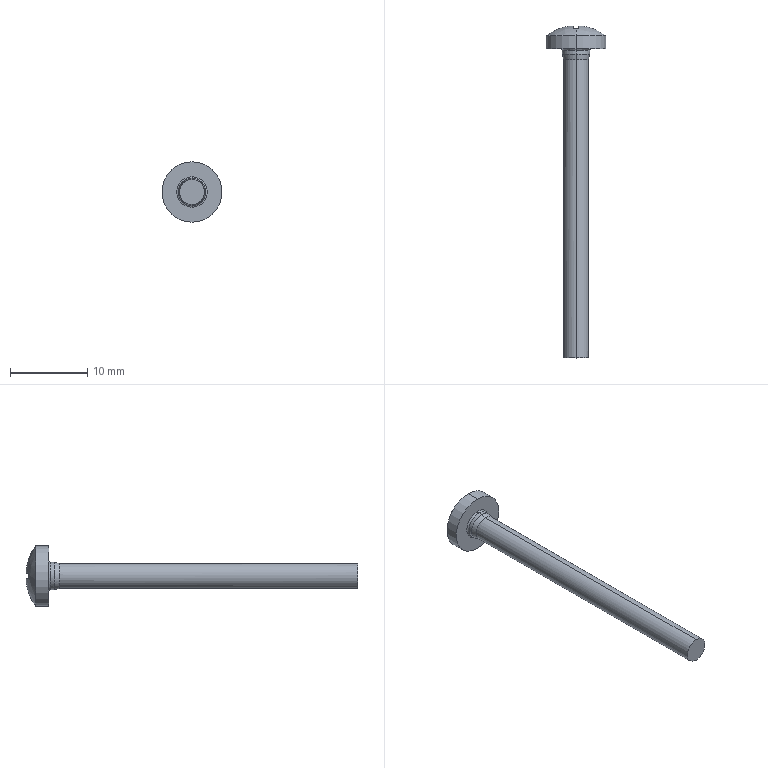Part | STEP file | 4-20.sldasm-Part-219 | 1 solid | 41 faces | box 7.82 x 42.968 x 7.82 mm | volume 439.236 mm3 | plane 18 | cone 8 | torus 7 | cylinder 6 | sphere 2 | commonest cylinder face diameters 3.241 x2 3.545 x2 7.82 x2
STEP:
#1=CARTESIAN_POINT('',(211.295,577.278,-21.679));
#2=VERTEX_POINT('',#1);
#3=CARTESIAN_POINT('',(211.295,577.278,-24.921));
#4=VERTEX_POINT('',#3);
#5=CARTESIAN_POINT('',(211.295,577.278,-23.3));
#6=DIRECTION('',(0.,-1.,0.));
#7=DIRECTION('',(0.,0.,1.));
#8=AXIS2_PLACEMENT_3D('',#5,#6,#7);
#9=CIRCLE('',#8,1.621);
#10=EDGE_CURVE('',#2,#4,#9,.T.);
#11=ORIENTED_EDGE('',*,*,#10,.F.);
#12=CARTESIAN_POINT('',(211.295,577.978,-21.528));
#13=VERTEX_POINT('',#12);
#14=CARTESIAN_POINT('',(211.295,577.278,-21.679));
#15=DIRECTION('',(0.,0.9775,0.2109));
#16=VECTOR('',#15,1000.);
#17=LINE('',#14,#16);
#18=EDGE_CURVE('',#2,#13,#17,.T.);
#19=ORIENTED_EDGE('',*,*,#18,.T.);
#20=CARTESIAN_POINT('',(211.295,577.978,-25.072));
#21=VERTEX_POINT('',#20);
#22=CARTESIAN_POINT('',(211.295,577.978,-21.528));
#23=CARTESIAN_POINT('',(211.063,577.978,-21.528));
#24=CARTESIAN_POINT('',(210.831,577.978,-21.574));
#25=CARTESIAN_POINT('',(210.403,577.978,-21.752));
#26=CARTESIAN_POINT('',(210.206,577.978,-21.883));
#27=CARTESIAN_POINT('',(209.878,577.978,-22.211));
#28=CARTESIAN_POINT('',(209.747,577.978,-22.408));
#29=CARTESIAN_POINT('',(209.569,577.978,-22.836));
#30=CARTESIAN_POINT('',(209.523,577.978,-23.068));
#31=CARTESIAN_POINT('',(209.523,577.978,-23.532));
#32=CARTESIAN_POINT('',(209.569,577.978,-23.764));
#33=CARTESIAN_POINT('',(209.747,577.978,-24.192));
#34=CARTESIAN_POINT('',(209.878,577.978,-24.389));
#35=CARTESIAN_POINT('',(210.206,577.978,-24.717));
#36=CARTESIAN_POINT('',(210.403,577.978,-24.848));
#37=CARTESIAN_POINT('',(210.831,577.978,-25.026));
#38=CARTESIAN_POINT('',(211.063,577.978,-25.072));
#39=CARTESIAN_POINT('',(211.295,577.978,-25.072));
#40=B_SPLINE_CURVE_WITH_KNOTS('',3,(#22,#23,#24,#25,#26,#27,#28,#29,#30,#31,#32,#33,#34,#35,#36,#37,#38,#39),.UNSPECIFIED.,.F.,.F.,(4,2,2,2,2,2,2,2,4),(0.,0.0625,0.125,0.1875,0.25,0.3125,0.375,0.4375,0.5),.UNSPECIFIED.);
#41=EDGE_CURVE('',#13,#21,#40,.T.);
#42=ORIENTED_EDGE('',*,*,#41,.T.);
#43=CARTESIAN_POINT('',(211.295,577.278,-24.921));
#44=DIRECTION('',(0.,0.9775,-0.2109));
#45=VECTOR('',#44,1000.);
#46=LINE('',#43,#45);
#47=EDGE_CURVE('',#4,#21,#46,.T.);
#48=ORIENTED_EDGE('',*,*,#47,.F.);
#49=EDGE_LOOP('',(#11,#19,#42,#48));
#50=FACE_OUTER_BOUND('',#49,.T.);
#51=CARTESIAN_POINT('',(211.295,577.278,-23.3));
#52=DIRECTION('',(0.,1.,0.));
#53=DIRECTION('',(0.,0.,-1.));
#54=AXIS2_PLACEMENT_3D('',#51,#52,#53);
#55=CONICAL_SURFACE('',#54,1.621,0.2125);
#56=ADVANCED_FACE('',(#50),#55,.T.);
#57=ORIENTED_EDGE('',*,*,#10,.T.);
#58=CARTESIAN_POINT('',(211.295,538.678,-24.921));
#59=VERTEX_POINT('',#58);
#60=CARTESIAN_POINT('',(211.295,577.278,-24.921));
#61=DIRECTION('',(0.,-1.,0.));
#62=VECTOR('',#61,1000.);
#63=LINE('',#60,#62);
#64=EDGE_CURVE('',#4,#59,#63,.T.);
#65=ORIENTED_EDGE('',*,*,#64,.T.);
#66=CARTESIAN_POINT('',(211.295,538.678,-21.679));
#67=VERTEX_POINT('',#66);
#68=CARTESIAN_POINT('',(211.295,538.678,-24.921));
#69=CARTESIAN_POINT('',(211.083,538.678,-24.921));
#70=CARTESIAN_POINT('',(210.871,538.678,-24.878));
#71=CARTESIAN_POINT('',(210.479,538.678,-24.716));
#72=CARTESIAN_POINT('',(210.299,538.678,-24.596));
#73=CARTESIAN_POINT('',(209.999,538.678,-24.296));
#74=CARTESIAN_POINT('',(209.879,538.678,-24.116));
#75=CARTESIAN_POINT('',(209.717,538.678,-23.724));
#76=CARTESIAN_POINT('',(209.674,538.678,-23.512));
#77=CARTESIAN_POINT('',(209.674,538.678,-23.088));
#78=CARTESIAN_POINT('',(209.717,538.678,-22.876));
#79=CARTESIAN_POINT('',(209.879,538.678,-22.484));
#80=CARTESIAN_POINT('',(209.999,538.678,-22.304));
#81=CARTESIAN_POINT('',(210.299,538.678,-22.004));
#82=CARTESIAN_POINT('',(210.479,538.678,-21.884));
#83=CARTESIAN_POINT('',(210.871,538.678,-21.722));
#84=CARTESIAN_POINT('',(211.083,538.678,-21.679));
#85=CARTESIAN_POINT('',(211.295,538.678,-21.679));
#86=B_SPLINE_CURVE_WITH_KNOTS('',3,(#68,#69,#70,#71,#72,#73,#74,#75,#76,#77,#78,#79,#80,#81,#82,#83,#84,#85),.UNSPECIFIED.,.F.,.F.,(4,2,2,2,2,2,2,2,4),(0.,0.0625,0.125,0.1875,0.25,0.3125,0.375,0.4375,0.5),.UNSPECIFIED.);
#87=EDGE_CURVE('',#59,#67,#86,.T.);
#88=ORIENTED_EDGE('',*,*,#87,.T.);
#89=CARTESIAN_POINT('',(211.295,577.278,-21.679));
#90=DIRECTION('',(0.,-1.,0.));
#91=VECTOR('',#90,1000.);
#92=LINE('',#89,#91);
#93=EDGE_CURVE('',#2,#67,#92,.T.);
#94=ORIENTED_EDGE('',*,*,#93,.F.);
#95=EDGE_LOOP('',(#57,#65,#88,#94));
#96=FACE_OUTER_BOUND('',#95,.T.);
#97=CARTESIAN_POINT('',(211.295,577.278,-23.3));
#98=DIRECTION('',(0.,-1.,0.));
#99=DIRECTION('',(0.,0.,1.));
#100=AXIS2_PLACEMENT_3D('',#97,#98,#99);
#101=CYLINDRICAL_SURFACE('',#100,1.621);
#102=ADVANCED_FACE('',(#96),#101,.T.);
#103=CARTESIAN_POINT('',(211.295,580.972,-21.744));
#104=VERTEX_POINT('',#103);
#105=CARTESIAN_POINT('',(211.661,580.972,-21.788));
#106=VERTEX_POINT('',#105);
#107=CARTESIAN_POINT('',(211.295,580.972,-23.3));
#108=DIRECTION('',(0.,1.,0.));
#109=DIRECTION('',(0.,0.,-1.));
#110=AXIS2_PLACEMENT_3D('',#107,#108,#109);
#111=CIRCLE('',#110,1.556);
#112=EDGE_CURVE('',#104,#106,#111,.T.);
#113=ORIENTED_EDGE('',*,*,#112,.F.);
#114=CARTESIAN_POINT('',(211.295,581.265,-20.994));
#115=VERTEX_POINT('',#114);
#116=CARTESIAN_POINT('',(211.295,580.704,-21.207));
#117=DIRECTION('',(1.,0.,0.));
#118=DIRECTION('',(0.,0.,-1.));
#119=AXIS2_PLACEMENT_3D('',#116,#117,#118);
#120=CIRCLE('',#119,0.6);
#121=EDGE_CURVE('',#104,#115,#120,.T.);
#122=ORIENTED_EDGE('',*,*,#121,.T.);
#123=CARTESIAN_POINT('',(211.648,581.265,-21.021));
#124=VERTEX_POINT('',#123);
#125=CARTESIAN_POINT('',(211.295,581.265,-23.3));
#126=DIRECTION('',(0.,-1.,0.));
#127=DIRECTION('',(0.,0.,1.));
#128=AXIS2_PLACEMENT_3D('',#125,#126,#127);
#129=CIRCLE('',#128,2.306);
#130=EDGE_CURVE('',#124,#115,#129,.T.);
#131=ORIENTED_EDGE('',*,*,#130,.F.);
#132=CARTESIAN_POINT('',(211.661,580.972,-21.788));
#133=CARTESIAN_POINT('',(211.66,581.106,-21.719));
#134=CARTESIAN_POINT('',(211.658,581.21,-21.6));
#135=CARTESIAN_POINT('',(211.653,581.317,-21.32));
#136=CARTESIAN_POINT('',(211.65,581.318,-21.163));
#137=CARTESIAN_POINT('',(211.648,581.265,-21.021));
#138=B_SPLINE_CURVE_WITH_KNOTS('',3,(#132,#133,#134,#135,#136,#137),.UNSPECIFIED.,.F.,.F.,(4,2,4),(0.,0.0004459,0.0008919),.UNSPECIFIED.);
#139=EDGE_CURVE('',#106,#124,#138,.T.);
#140=ORIENTED_EDGE('',*,*,#139,.F.);
#141=EDGE_LOOP('',(#113,#122,#131,#140));
#142=FACE_OUTER_BOUND('',#141,.T.);
#143=CARTESIAN_POINT('',(211.295,580.704,-23.3));
#144=DIRECTION('',(0.,-1.,0.));
#145=DIRECTION('',(0.,0.,1.));
#146=AXIS2_PLACEMENT_3D('',#143,#144,#145);
#147=TOROIDAL_SURFACE('',#146,2.093,0.6);
#148=ADVANCED_FACE('',(#142),#147,.T.);
#149=CARTESIAN_POINT('',(211.295,579.538,-23.3));
#150=VERTEX_POINT('',#149);
#151=CARTESIAN_POINT('',(210.775,579.93,-23.82));
#152=VERTEX_POINT('',#151);
#153=CARTESIAN_POINT('',(211.295,579.538,-23.3));
#154=DIRECTION('',(-0.6241,0.4702,-0.6241));
#155=VECTOR('',#154,1000.);
#156=LINE('',#153,#155);
#157=EDGE_CURVE('',#150,#152,#156,.T.);
#158=ORIENTED_EDGE('',*,*,#157,.F.);
#159=CARTESIAN_POINT('',(211.815,579.93,-22.78));
#160=VERTEX_POINT('',#159);
#161=CARTESIAN_POINT('',(211.295,579.538,-23.3));
#162=DIRECTION('',(0.6241,0.4702,0.6241));
#163=VECTOR('',#162,1000.);
#164=LINE('',#161,#163);
#165=EDGE_CURVE('',#150,#160,#164,.T.);
#166=ORIENTED_EDGE('',*,*,#165,.T.);
#167=CARTESIAN_POINT('',(212.119,580.021,-22.922));
#168=VERTEX_POINT('',#167);
#169=CARTESIAN_POINT('',(212.119,580.021,-22.922));
#170=CARTESIAN_POINT('',(212.019,579.983,-22.876));
#171=CARTESIAN_POINT('',(211.918,579.95,-22.829));
#172=CARTESIAN_POINT('',(211.815,579.93,-22.78));
#173=B_SPLINE_CURVE_WITH_KNOTS('',3,(#169,#170,#171,#172),.UNSPECIFIED.,.F.,.F.,(4,4),(0.000000233,0.0003479),.UNSPECIFIED.);
#174=EDGE_CURVE('',#168,#160,#173,.T.);
#175=ORIENTED_EDGE('',*,*,#174,.F.);
#176=CARTESIAN_POINT('',(212.377,580.148,-22.927));
#177=VERTEX_POINT('',#176);
#178=CARTESIAN_POINT('',(212.377,580.148,-22.927));
#179=CARTESIAN_POINT('',(212.292,580.105,-22.925));
#180=CARTESIAN_POINT('',(212.205,580.062,-22.924));
#181=CARTESIAN_POINT('',(212.119,580.021,-22.922));
#182=B_SPLINE_CURVE_WITH_KNOTS('',3,(#178,#179,#180,#181),.UNSPECIFIED.,.F.,.F.,(4,4),(0.000000447,0.0002887),.UNSPECIFIED.);
#183=EDGE_CURVE('',#177,#168,#182,.T.);
#184=ORIENTED_EDGE('',*,*,#183,.F.);
#185=CARTESIAN_POINT('',(212.377,580.148,-23.673));
#186=VERTEX_POINT('',#185);
#187=CARTESIAN_POINT('',(211.295,580.148,-23.3));
#188=DIRECTION('',(0.,-1.,0.));
#189=DIRECTION('',(0.7071,0.,0.7071));
#190=AXIS2_PLACEMENT_3D('',#187,#188,#189);
#191=CIRCLE('',#190,1.145);
#192=EDGE_CURVE('',#186,#177,#191,.T.);
#193=ORIENTED_EDGE('',*,*,#192,.F.);
#194=CARTESIAN_POINT('',(212.119,580.021,-23.678));
#195=VERTEX_POINT('',#194);
#196=CARTESIAN_POINT('',(212.119,580.021,-23.678));
#197=CARTESIAN_POINT('',(212.205,580.062,-23.676));
#198=CARTESIAN_POINT('',(212.292,580.105,-23.675));
#199=CARTESIAN_POINT('',(212.377,580.148,-23.673));
#200=B_SPLINE_CURVE_WITH_KNOTS('',3,(#196,#197,#198,#199),.UNSPECIFIED.,.F.,.F.,(4,4),(0.000000222,0.0002885),.UNSPECIFIED.);
#201=EDGE_CURVE('',#195,#186,#200,.T.);
#202=ORIENTED_EDGE('',*,*,#201,.F.);
#203=CARTESIAN_POINT('',(211.815,579.93,-23.82));
#204=VERTEX_POINT('',#203);
#205=CARTESIAN_POINT('',(211.815,579.93,-23.82));
#206=CARTESIAN_POINT('',(211.918,579.95,-23.771));
#207=CARTESIAN_POINT('',(212.019,579.983,-23.724));
#208=CARTESIAN_POINT('',(212.119,580.021,-23.678));
#209=B_SPLINE_CURVE_WITH_KNOTS('',3,(#205,#206,#207,#208),.UNSPECIFIED.,.F.,.F.,(4,4),(0.000000224,0.0003479),.UNSPECIFIED.);
#210=EDGE_CURVE('',#204,#195,#209,.T.);
#211=ORIENTED_EDGE('',*,*,#210,.F.);
#212=CARTESIAN_POINT('',(211.673,580.021,-24.124));
#213=VERTEX_POINT('',#212);
#214=CARTESIAN_POINT('',(211.673,580.021,-24.124));
#215=CARTESIAN_POINT('',(211.719,579.983,-24.024));
#216=CARTESIAN_POINT('',(211.766,579.95,-23.923));
#217=CARTESIAN_POINT('',(211.815,579.93,-23.82));
#218=B_SPLINE_CURVE_WITH_KNOTS('',3,(#214,#215,#216,#217),.UNSPECIFIED.,.F.,.F.,(4,4),(0.000000233,0.0003479),.UNSPECIFIED.);
#219=EDGE_CURVE('',#213,#204,#218,.T.);
#220=ORIENTED_EDGE('',*,*,#219,.F.);
#221=CARTESIAN_POINT('',(211.668,580.148,-24.382));
#222=VERTEX_POINT('',#221);
#223=CARTESIAN_POINT('',(211.668,580.148,-24.382));
#224=CARTESIAN_POINT('',(211.67,580.105,-24.296));
#225=CARTESIAN_POINT('',(211.671,580.062,-24.21));
#226=CARTESIAN_POINT('',(211.673,580.021,-24.124));
#227=B_SPLINE_CURVE_WITH_KNOTS('',3,(#223,#224,#225,#226),.UNSPECIFIED.,.F.,.F.,(4,4),(0.000000447,0.0002887),.UNSPECIFIED.);
#228=EDGE_CURVE('',#222,#213,#227,.T.);
#229=ORIENTED_EDGE('',*,*,#228,.F.);
#230=CARTESIAN_POINT('',(210.922,580.148,-24.382));
#231=VERTEX_POINT('',#230);
#232=CARTESIAN_POINT('',(211.295,580.148,-23.3));
#233=DIRECTION('',(0.,-1.,0.));
#234=DIRECTION('',(0.7071,0.,0.7071));
#235=AXIS2_PLACEMENT_3D('',#232,#233,#234);
#236=CIRCLE('',#235,1.145);
#237=EDGE_CURVE('',#231,#222,#236,.T.);
#238=ORIENTED_EDGE('',*,*,#237,.F.);
#239=CARTESIAN_POINT('',(210.917,580.021,-24.124));
#240=VERTEX_POINT('',#239);
#241=CARTESIAN_POINT('',(210.917,580.021,-24.124));
#242=CARTESIAN_POINT('',(210.919,580.062,-24.21));
#243=CARTESIAN_POINT('',(210.92,580.105,-24.296));
#244=CARTESIAN_POINT('',(210.922,580.148,-24.382));
#245=B_SPLINE_CURVE_WITH_KNOTS('',3,(#241,#242,#243,#244),.UNSPECIFIED.,.F.,.F.,(4,4),(0.000000222,0.0002885),.UNSPECIFIED.);
#246=EDGE_CURVE('',#240,#231,#245,.T.);
#247=ORIENTED_EDGE('',*,*,#246,.F.);
#248=CARTESIAN_POINT('',(210.775,579.93,-23.82));
#249=CARTESIAN_POINT('',(210.824,579.95,-23.923));
#250=CARTESIAN_POINT('',(210.871,579.983,-24.024));
#251=CARTESIAN_POINT('',(210.917,580.021,-24.124));
#252=B_SPLINE_CURVE_WITH_KNOTS('',3,(#248,#249,#250,#251),.UNSPECIFIED.,.F.,.F.,(4,4),(0.000000224,0.0003479),.UNSPECIFIED.);
#253=EDGE_CURVE('',#152,#240,#252,.T.);
#254=ORIENTED_EDGE('',*,*,#253,.F.);
#255=EDGE_LOOP('',(#158,#166,#175,#184,#193,#202,#211,#220,#229,#238,#247,#254));
#256=FACE_OUTER_BOUND('',#255,.T.);
#257=CARTESIAN_POINT('',(211.295,1579.538,-23.3));
#258=DIRECTION('',(0.,1.,0.));
#259=DIRECTION('',(-0.7071,0.,-0.7071));
#260=AXIS2_PLACEMENT_3D('',#257,#258,#259);
#261=CONICAL_SURFACE('',#260,1877.049,1.081);
#262=ADVANCED_FACE('',(#256),#261,.F.);
#263=CARTESIAN_POINT('',(211.295,578.478,-25.073));
#264=VERTEX_POINT('',#263);
#265=CARTESIAN_POINT('',(211.295,578.478,-21.527));
#266=VERTEX_POINT('',#265);
#267=CARTESIAN_POINT('',(211.295,578.478,-23.3));
#268=DIRECTION('',(0.,-1.,0.));
#269=DIRECTION('',(0.,0.,1.));
#270=AXIS2_PLACEMENT_3D('',#267,#268,#269);
#271=CIRCLE('',#270,1.773);
#272=EDGE_CURVE('',#264,#266,#271,.T.);
#273=ORIENTED_EDGE('',*,*,#272,.F.);
#274=CARTESIAN_POINT('',(211.295,578.678,-25.273));
#275=VERTEX_POINT('',#274);
#276=CARTESIAN_POINT('',(211.295,578.478,-25.273));
#277=DIRECTION('',(-1.,0.,0.));
#278=DIRECTION('',(0.,0.,1.));
#279=AXIS2_PLACEMENT_3D('',#276,#277,#278);
#280=CIRCLE('',#279,0.2);
#281=EDGE_CURVE('',#264,#275,#280,.T.);
#282=ORIENTED_EDGE('',*,*,#281,.T.);
#283=CARTESIAN_POINT('',(211.295,578.678,-21.327));
#284=VERTEX_POINT('',#283);
#285=CARTESIAN_POINT('',(211.295,578.678,-23.3));
#286=DIRECTION('',(0.,1.,0.));
#287=DIRECTION('',(0.,0.,1.));
#288=AXIS2_PLACEMENT_3D('',#285,#286,#287);
#289=CIRCLE('',#288,1.973);
#290=EDGE_CURVE('',#284,#275,#289,.T.);
#291=ORIENTED_EDGE('',*,*,#290,.F.);
#292=CARTESIAN_POINT('',(211.295,578.478,-21.327));
#293=DIRECTION('',(1.,0.,0.));
#294=DIRECTION('',(0.,0.,-1.));
#295=AXIS2_PLACEMENT_3D('',#292,#293,#294);
#296=CIRCLE('',#295,0.2);
#297=EDGE_CURVE('',#266,#284,#296,.T.);
#298=ORIENTED_EDGE('',*,*,#297,.F.);
#299=EDGE_LOOP('',(#273,#282,#291,#298));
#300=FACE_OUTER_BOUND('',#299,.T.);
#301=CARTESIAN_POINT('',(211.295,578.478,-23.3));
#302=DIRECTION('',(0.,-1.,0.));
#303=DIRECTION('',(0.,0.,1.));
#304=AXIS2_PLACEMENT_3D('',#301,#302,#303);
#305=TOROIDAL_SURFACE('',#304,1.973,0.2);
#306=ADVANCED_FACE('',(#300),#305,.F.);
#307=CARTESIAN_POINT('',(211.295,578.478,-23.3));
#308=DIRECTION('',(0.,-1.,0.));
#309=DIRECTION('',(0.,0.,1.));
#310=AXIS2_PLACEMENT_3D('',#307,#308,#309);
#311=CIRCLE('',#310,1.773);
#312=EDGE_CURVE('',#266,#264,#311,.T.);
#313=ORIENTED_EDGE('',*,*,#312,.T.);
#314=CARTESIAN_POINT('',(211.295,578.678,-25.073));
#315=DIRECTION('',(0.,-1.,0.));
#316=VECTOR('',#315,1000.);
#317=LINE('',#314,#316);
#318=EDGE_CURVE('',#264,#21,#317,.T.);
#319=ORIENTED_EDGE('',*,*,#318,.T.);
#320=ORIENTED_EDGE('',*,*,#41,.F.);
#321=CARTESIAN_POINT('',(211.295,578.678,-21.527));
#322=DIRECTION('',(0.,-1.,0.));
#323=VECTOR('',#322,1000.);
#324=LINE('',#321,#323);
#325=EDGE_CURVE('',#266,#13,#324,.T.);
#326=ORIENTED_EDGE('',*,*,#325,.F.);
#327=EDGE_LOOP('',(#313,#319,#320,#326));
#328=FACE_OUTER_BOUND('',#327,.T.);
#329=CARTESIAN_POINT('',(211.295,578.678,-23.3));
#330=DIRECTION('',(0.,-1.,0.));
#331=DIRECTION('',(0.,0.,1.));
#332=AXIS2_PLACEMENT_3D('',#329,#330,#331);
#333=CYLINDRICAL_SURFACE('',#332,1.773);
#334=ADVANCED_FACE('',(#328),#333,.T.);
#335=CARTESIAN_POINT('',(211.295,580.38,-27.21));
#336=VERTEX_POINT('',#335);
#337=CARTESIAN_POINT('',(211.295,580.38,-19.39));
#338=VERTEX_POINT('',#337);
#339=CARTESIAN_POINT('',(211.295,580.38,-23.3));
#340=DIRECTION('',(0.,1.,0.));
#341=DIRECTION('',(0.,0.,1.));
#342=AXIS2_PLACEMENT_3D('',#339,#340,#341);
#343=CIRCLE('',#342,3.91);
#344=EDGE_CURVE('',#336,#338,#343,.T.);
#345=ORIENTED_EDGE('',*,*,#344,.T.);
#346=CARTESIAN_POINT('',(211.295,575.188,-23.3));
#347=DIRECTION('',(-1.,0.,0.));
#348=DIRECTION('',(0.,0.,1.));
#349=AXIS2_PLACEMENT_3D('',#346,#347,#348);
#350=CIRCLE('',#349,6.5);
#351=EDGE_CURVE('',#338,#115,#350,.T.);
#352=ORIENTED_EDGE('',*,*,#351,.T.);
#353=CARTESIAN_POINT('',(210.942,581.265,-21.021));
#354=VERTEX_POINT('',#353);
#355=CARTESIAN_POINT('',(211.295,581.265,-23.3));
#356=DIRECTION('',(0.,-1.,0.));
#357=DIRECTION('',(0.,0.,1.));
#358=AXIS2_PLACEMENT_3D('',#355,#356,#357);
#359=CIRCLE('',#358,2.306);
#360=EDGE_CURVE('',#115,#354,#359,.T.);
#361=ORIENTED_EDGE('',*,*,#360,.T.);
#362=CARTESIAN_POINT('',(210.917,581.625,-22.476));
#363=VERTEX_POINT('',#362);
#364=CARTESIAN_POINT('',(210.903,575.188,-23.293));
#365=DIRECTION('',(0.9998,0.,-0.01745));
#366=DIRECTION('',(0.01745,0.,0.9998));
#367=AXIS2_PLACEMENT_3D('',#364,#365,#366);
#368=CIRCLE('',#367,6.488);
#369=EDGE_CURVE('',#363,#354,#368,.T.);
#370=ORIENTED_EDGE('',*,*,#369,.F.);
#371=CARTESIAN_POINT('',(210.775,581.646,-22.78));
#372=VERTEX_POINT('',#371);
#373=CARTESIAN_POINT('',(210.669,575.188,-23.008));
#374=DIRECTION('',(0.9063,0.,-0.4226));
#375=DIRECTION('',(0.4226,0.,0.9063));
#376=AXIS2_PLACEMENT_3D('',#373,#374,#375);
#377=CIRCLE('',#376,6.463);
#378=EDGE_CURVE('',#372,#363,#377,.T.);
#379=ORIENTED_EDGE('',*,*,#378,.F.);
#380=CARTESIAN_POINT('',(210.471,581.625,-22.922));
#381=VERTEX_POINT('',#380);
#382=CARTESIAN_POINT('',(211.003,575.188,-22.674));
#383=DIRECTION('',(0.4226,0.,-0.9063));
#384=DIRECTION('',(0.9063,0.,0.4226));
#385=AXIS2_PLACEMENT_3D('',#382,#383,#384);
#386=CIRCLE('',#385,6.463);
#387=EDGE_CURVE('',#381,#372,#386,.T.);
#388=ORIENTED_EDGE('',*,*,#387,.F.);
#389=CARTESIAN_POINT('',(209.016,581.265,-22.947));
#390=VERTEX_POINT('',#389);
#391=CARTESIAN_POINT('',(211.288,575.188,-22.908));
#392=DIRECTION('',(0.01745,0.,-0.9998));
#393=DIRECTION('',(0.9998,0.,0.01745));
#394=AXIS2_PLACEMENT_3D('',#391,#392,#393);
#395=CIRCLE('',#394,6.488);
#396=EDGE_CURVE('',#390,#381,#395,.T.);
#397=ORIENTED_EDGE('',*,*,#396,.F.);
#398=CARTESIAN_POINT('',(209.016,581.265,-23.653));
#399=VERTEX_POINT('',#398);
#400=CARTESIAN_POINT('',(211.295,581.265,-23.3));
#401=DIRECTION('',(0.,-1.,0.));
#402=DIRECTION('',(0.,0.,1.));
#403=AXIS2_PLACEMENT_3D('',#400,#401,#402);
#404=CIRCLE('',#403,2.306);
#405=EDGE_CURVE('',#390,#399,#404,.T.);
#406=ORIENTED_EDGE('',*,*,#405,.T.);
#407=CARTESIAN_POINT('',(210.471,581.625,-23.678));
#408=VERTEX_POINT('',#407);
#409=CARTESIAN_POINT('',(211.288,575.188,-23.692));
#410=DIRECTION('',(0.01745,0.,0.9998));
#411=DIRECTION('',(-0.9998,0.,0.01745));
#412=AXIS2_PLACEMENT_3D('',#409,#410,#411);
#413=CIRCLE('',#412,6.488);
#414=EDGE_CURVE('',#408,#399,#413,.T.);
#415=ORIENTED_EDGE('',*,*,#414,.F.);
#416=CARTESIAN_POINT('',(210.775,581.646,-23.82));
#417=VERTEX_POINT('',#416);
#418=CARTESIAN_POINT('',(211.003,575.188,-23.926));
#419=DIRECTION('',(0.4226,0.,0.9063));
#420=DIRECTION('',(-0.9063,0.,0.4226));
#421=AXIS2_PLACEMENT_3D('',#418,#419,#420);
#422=CIRCLE('',#421,6.463);
#423=EDGE_CURVE('',#417,#408,#422,.T.);
#424=ORIENTED_EDGE('',*,*,#423,.F.);
#425=CARTESIAN_POINT('',(210.917,581.625,-24.124));
#426=VERTEX_POINT('',#425);
#427=CARTESIAN_POINT('',(210.669,575.188,-23.592));
#428=DIRECTION('',(0.9063,0.,0.4226));
#429=DIRECTION('',(-0.4226,0.,0.9063));
#430=AXIS2_PLACEMENT_3D('',#427,#428,#429);
#431=CIRCLE('',#430,6.463);
#432=EDGE_CURVE('',#426,#417,#431,.T.);
#433=ORIENTED_EDGE('',*,*,#432,.F.);
#434=CARTESIAN_POINT('',(210.942,581.265,-25.579));
#435=VERTEX_POINT('',#434);
#436=CARTESIAN_POINT('',(210.903,575.188,-23.307));
#437=DIRECTION('',(0.9998,0.,0.01745));
#438=DIRECTION('',(-0.01745,0.,0.9998));
#439=AXIS2_PLACEMENT_3D('',#436,#437,#438);
#440=CIRCLE('',#439,6.488);
#441=EDGE_CURVE('',#435,#426,#440,.T.);
#442=ORIENTED_EDGE('',*,*,#441,.F.);
#443=CARTESIAN_POINT('',(211.295,581.265,-25.606));
#444=VERTEX_POINT('',#443);
#445=CARTESIAN_POINT('',(211.295,581.265,-23.3));
#446=DIRECTION('',(0.,-1.,0.));
#447=DIRECTION('',(0.,0.,1.));
#448=AXIS2_PLACEMENT_3D('',#445,#446,#447);
#449=CIRCLE('',#448,2.306);
#450=EDGE_CURVE('',#435,#444,#449,.T.);
#451=ORIENTED_EDGE('',*,*,#450,.T.);
#452=CARTESIAN_POINT('',(211.295,575.188,-23.3));
#453=DIRECTION('',(1.,0.,0.));
#454=DIRECTION('',(0.,0.,-1.));
#455=AXIS2_PLACEMENT_3D('',#452,#453,#454);
#456=CIRCLE('',#455,6.5);
#457=EDGE_CURVE('',#336,#444,#456,.T.);
#458=ORIENTED_EDGE('',*,*,#457,.F.);
#459=EDGE_LOOP('',(#345,#352,#361,#370,#379,#388,#397,#406,#415,#424,#433,#442,#451,#458));
#460=FACE_OUTER_BOUND('',#459,.T.);
#461=CARTESIAN_POINT('',(211.295,575.188,-23.3));
#462=DIRECTION('',(-1.,0.,0.));
#463=DIRECTION('',(0.,0.,-1.));
#464=AXIS2_PLACEMENT_3D('',#461,#462,#463);
#465=SPHERICAL_SURFACE('',#464,6.5);
#466=ADVANCED_FACE('',(#460),#465,.T.);
#467=ORIENTED_EDGE('',*,*,#344,.F.);
#468=CARTESIAN_POINT('',(211.295,578.678,-27.21));
#469=VERTEX_POINT('',#468);
#470=CARTESIAN_POINT('',(211.295,581.688,-27.21));
#471=DIRECTION('',(0.,-1.,0.));
#472=VECTOR('',#471,1000.);
#473=LINE('',#470,#472);
#474=EDGE_CURVE('',#336,#469,#473,.T.);
#475=ORIENTED_EDGE('',*,*,#474,.T.);
#476=CARTESIAN_POINT('',(211.295,578.678,-19.39));
#477=VERTEX_POINT('',#476);
#478=CARTESIAN_POINT('',(211.295,578.678,-23.3));
#479=DIRECTION('',(0.,1.,0.));
#480=DIRECTION('',(0.,0.,-1.));
#481=AXIS2_PLACEMENT_3D('',#478,#479,#480);
#482=CIRCLE('',#481,3.91);
#483=EDGE_CURVE('',#469,#477,#482,.T.);
#484=ORIENTED_EDGE('',*,*,#483,.T.);
#485=CARTESIAN_POINT('',(211.295,581.688,-19.39));
#486=DIRECTION('',(0.,-1.,0.));
#487=VECTOR('',#486,1000.);
#488=LINE('',#485,#487);
#489=EDGE_CURVE('',#338,#477,#488,.T.);
#490=ORIENTED_EDGE('',*,*,#489,.F.);
#491=EDGE_LOOP('',(#467,#475,#484,#490));
#492=FACE_OUTER_BOUND('',#491,.T.);
#493=CARTESIAN_POINT('',(211.295,581.688,-23.3));
#494=DIRECTION('',(0.,-1.,0.));
#495=DIRECTION('',(0.,0.,1.));
#496=AXIS2_PLACEMENT_3D('',#493,#494,#495);
#497=CYLINDRICAL_SURFACE('',#496,3.91);
#498=ADVANCED_FACE('',(#492),#497,.T.);
#499=ORIENTED_EDGE('',*,*,#290,.T.);
#500=CARTESIAN_POINT('',(211.295,578.678,-23.3));
#501=DIRECTION('',(0.,1.,0.));
#502=DIRECTION('',(0.,0.,1.));
#503=AXIS2_PLACEMENT_3D('',#500,#501,#502);
#504=CIRCLE('',#503,1.973);
#505=EDGE_CURVE('',#275,#284,#504,.T.);
#506=ORIENTED_EDGE('',*,*,#505,.T.);
#507=EDGE_LOOP('',(#499,#506));
#508=FACE_BOUND('',#507,.T.);
#509=CARTESIAN_POINT('',(211.295,578.678,-23.3));
#510=DIRECTION('',(0.,1.,0.));
#511=DIRECTION('',(0.,0.,-1.));
#512=AXIS2_PLACEMENT_3D('',#509,#510,#511);
#513=CIRCLE('',#512,3.91);
#514=EDGE_CURVE('',#477,#469,#513,.T.);
#515=ORIENTED_EDGE('',*,*,#514,.F.);
#516=ORIENTED_EDGE('',*,*,#483,.F.);
#517=EDGE_LOOP('',(#515,#516));
#518=FACE_OUTER_BOUND('',#517,.T.);
#519=CARTESIAN_POINT('',(211.295,578.678,-23.3));
#520=DIRECTION('',(0.,-1.,0.));
#521=DIRECTION('',(0.,0.,1.));
#522=AXIS2_PLACEMENT_3D('',#519,#520,#521);
#523=PLANE('',#522);
#524=ADVANCED_FACE('',(#508,#518),#523,.T.);
#525=ORIENTED_EDGE('',*,*,#474,.F.);
#526=CARTESIAN_POINT('',(211.295,580.38,-23.3));
#527=DIRECTION('',(0.,1.,0.));
#528=DIRECTION('',(0.,0.,1.));
#529=AXIS2_PLACEMENT_3D('',#526,#527,#528);
#530=CIRCLE('',#529,3.91);
#531=EDGE_CURVE('',#338,#336,#530,.T.);
#532=ORIENTED_EDGE('',*,*,#531,.F.);
#533=ORIENTED_EDGE('',*,*,#489,.T.);
#534=ORIENTED_EDGE('',*,*,#514,.T.);
#535=EDGE_LOOP('',(#525,#532,#533,#534));
#536=FACE_OUTER_BOUND('',#535,.T.);
#537=CARTESIAN_POINT('',(211.295,581.688,-23.3));
#538=DIRECTION('',(0.,-1.,0.));
#539=DIRECTION('',(0.,0.,1.));
#540=AXIS2_PLACEMENT_3D('',#537,#538,#539);
#541=CYLINDRICAL_SURFACE('',#540,3.91);
#542=ADVANCED_FACE('',(#536),#541,.T.);
#543=ORIENTED_EDGE('',*,*,#351,.F.);
#544=ORIENTED_EDGE('',*,*,#531,.T.);
#545=ORIENTED_EDGE('',*,*,#457,.T.);
#546=CARTESIAN_POINT('',(211.648,581.265,-25.579));
#547=VERTEX_POINT('',#546);
#548=CARTESIAN_POINT('',(211.295,581.265,-23.3));
#549=DIRECTION('',(0.,-1.,0.));
#550=DIRECTION('',(0.,0.,1.));
#551=AXIS2_PLACEMENT_3D('',#548,#549,#550);
#552=CIRCLE('',#551,2.306);
#553=EDGE_CURVE('',#444,#547,#552,.T.);
#554=ORIENTED_EDGE('',*,*,#553,.T.);
#555=CARTESIAN_POINT('',(211.673,581.625,-24.124));
#556=VERTEX_POINT('',#555);
#557=CARTESIAN_POINT('',(211.687,575.188,-23.307));
#558=DIRECTION('',(-0.9998,0.,0.01745));
#559=DIRECTION('',(-0.01745,0.,-0.9998));
#560=AXIS2_PLACEMENT_3D('',#557,#558,#559);
#561=CIRCLE('',#560,6.488);
#562=EDGE_CURVE('',#556,#547,#561,.T.);
#563=ORIENTED_EDGE('',*,*,#562,.F.);
#564=CARTESIAN_POINT('',(211.815,581.646,-23.82));
#565=VERTEX_POINT('',#564);
#566=CARTESIAN_POINT('',(211.921,575.188,-23.592));
#567=DIRECTION('',(-0.9063,0.,0.4226));
#568=DIRECTION('',(-0.4226,0.,-0.9063));
#569=AXIS2_PLACEMENT_3D('',#566,#567,#568);
#570=CIRCLE('',#569,6.463);
#571=EDGE_CURVE('',#565,#556,#570,.T.);
#572=ORIENTED_EDGE('',*,*,#571,.F.);
#573=CARTESIAN_POINT('',(212.119,581.625,-23.678));
#574=VERTEX_POINT('',#573);
#575=CARTESIAN_POINT('',(211.587,575.188,-23.926));
#576=DIRECTION('',(-0.4226,0.,0.9063));
#577=DIRECTION('',(-0.9063,0.,-0.4226));
#578=AXIS2_PLACEMENT_3D('',#575,#576,#577);
#579=CIRCLE('',#578,6.463);
#580=EDGE_CURVE('',#574,#565,#579,.T.);
#581=ORIENTED_EDGE('',*,*,#580,.F.);
#582=CARTESIAN_POINT('',(213.574,581.265,-23.653));
#583=VERTEX_POINT('',#582);
#584=CARTESIAN_POINT('',(211.302,575.188,-23.692));
#585=DIRECTION('',(-0.01745,0.,0.9998));
#586=DIRECTION('',(-0.9998,0.,-0.01745));
#587=AXIS2_PLACEMENT_3D('',#584,#585,#586);
#588=CIRCLE('',#587,6.488);
#589=EDGE_CURVE('',#583,#574,#588,.T.);
#590=ORIENTED_EDGE('',*,*,#589,.F.);
#591=CARTESIAN_POINT('',(213.574,581.265,-22.947));
#592=VERTEX_POINT('',#591);
#593=CARTESIAN_POINT('',(211.295,581.265,-23.3));
#594=DIRECTION('',(0.,-1.,0.));
#595=DIRECTION('',(0.,0.,1.));
#596=AXIS2_PLACEMENT_3D('',#593,#594,#595);
#597=CIRCLE('',#596,2.306);
#598=EDGE_CURVE('',#583,#592,#597,.T.);
#599=ORIENTED_EDGE('',*,*,#598,.T.);
#600=CARTESIAN_POINT('',(212.119,581.625,-22.922));
#601=VERTEX_POINT('',#600);
#602=CARTESIAN_POINT('',(211.302,575.188,-22.908));
#603=DIRECTION('',(-0.01745,0.,-0.9998));
#604=DIRECTION('',(0.9998,0.,-0.01745));
#605=AXIS2_PLACEMENT_3D('',#602,#603,#604);
#606=CIRCLE('',#605,6.488);
#607=EDGE_CURVE('',#601,#592,#606,.T.);
#608=ORIENTED_EDGE('',*,*,#607,.F.);
#609=CARTESIAN_POINT('',(211.815,581.646,-22.78));
#610=VERTEX_POINT('',#609);
#611=CARTESIAN_POINT('',(211.587,575.188,-22.674));
#612=DIRECTION('',(-0.4226,0.,-0.9063));
#613=DIRECTION('',(0.9063,0.,-0.4226));
#614=AXIS2_PLACEMENT_3D('',#611,#612,#613);
#615=CIRCLE('',#614,6.463);
#616=EDGE_CURVE('',#610,#601,#615,.T.);
#617=ORIENTED_EDGE('',*,*,#616,.F.);
#618=CARTESIAN_POINT('',(211.673,581.625,-22.476));
#619=VERTEX_POINT('',#618);
#620=CARTESIAN_POINT('',(211.921,575.188,-23.008));
#621=DIRECTION('',(-0.9063,0.,-0.4226));
#622=DIRECTION('',(0.4226,0.,-0.9063));
#623=AXIS2_PLACEMENT_3D('',#620,#621,#622);
#624=CIRCLE('',#623,6.463);
#625=EDGE_CURVE('',#619,#610,#624,.T.);
#626=ORIENTED_EDGE('',*,*,#625,.F.);
#627=CARTESIAN_POINT('',(211.687,575.188,-23.293));
#628=DIRECTION('',(-0.9998,0.,-0.01745));
#629=DIRECTION('',(0.01745,0.,-0.9998));
#630=AXIS2_PLACEMENT_3D('',#627,#628,#629);
#631=CIRCLE('',#630,6.488);
#632=EDGE_CURVE('',#124,#619,#631,.T.);
#633=ORIENTED_EDGE('',*,*,#632,.F.);
#634=ORIENTED_EDGE('',*,*,#130,.T.);
#635=EDGE_LOOP('',(#543,#544,#545,#554,#563,#572,#581,#590,#599,#608,#617,#626,#633,#634));
#636=FACE_OUTER_BOUND('',#635,.T.);
#637=CARTESIAN_POINT('',(211.295,575.188,-23.3));
#638=DIRECTION('',(-1.,0.,0.));
#639=DIRECTION('',(0.,0.,-1.));
#640=AXIS2_PLACEMENT_3D('',#637,#638,#639);
#641=SPHERICAL_SURFACE('',#640,6.5);
#642=ADVANCED_FACE('',(#636),#641,.T.);
#643=ORIENTED_EDGE('',*,*,#318,.F.);
#644=ORIENTED_EDGE('',*,*,#272,.T.);
#645=ORIENTED_EDGE('',*,*,#325,.T.);
#646=CARTESIAN_POINT('',(211.295,577.978,-25.072));
#647=CARTESIAN_POINT('',(211.527,577.978,-25.072));
#648=CARTESIAN_POINT('',(211.759,577.978,-25.026));
#649=CARTESIAN_POINT('',(212.187,577.978,-24.848));
#650=CARTESIAN_POINT('',(212.384,577.978,-24.717));
#651=CARTESIAN_POINT('',(212.712,577.978,-24.389));
#652=CARTESIAN_POINT('',(212.843,577.978,-24.192));
#653=CARTESIAN_POINT('',(213.021,577.978,-23.764));
#654=CARTESIAN_POINT('',(213.067,577.978,-23.532));
#655=CARTESIAN_POINT('',(213.067,577.978,-23.068));
#656=CARTESIAN_POINT('',(213.021,577.978,-22.836));
#657=CARTESIAN_POINT('',(212.843,577.978,-22.408));
#658=CARTESIAN_POINT('',(212.712,577.978,-22.211));
#659=CARTESIAN_POINT('',(212.384,577.978,-21.883));
#660=CARTESIAN_POINT('',(212.187,577.978,-21.752));
#661=CARTESIAN_POINT('',(211.759,577.978,-21.574));
#662=CARTESIAN_POINT('',(211.527,577.978,-21.528));
#663=CARTESIAN_POINT('',(211.295,577.978,-21.528));
#664=B_SPLINE_CURVE_WITH_KNOTS('',3,(#646,#647,#648,#649,#650,#651,#652,#653,#654,#655,#656,#657,#658,#659,#660,#661,#662,#663),.UNSPECIFIED.,.F.,.F.,(4,2,2,2,2,2,2,2,4),(0.5,0.5625,0.625,0.6875,0.75,0.8125,0.875,0.9375,1.),.UNSPECIFIED.);
#665=EDGE_CURVE('',#21,#13,#664,.T.);
#666=ORIENTED_EDGE('',*,*,#665,.F.);
#667=EDGE_LOOP('',(#643,#644,#645,#666));
#668=FACE_OUTER_BOUND('',#667,.T.);
#669=CARTESIAN_POINT('',(211.295,578.678,-23.3));
#670=DIRECTION('',(0.,-1.,0.));
#671=DIRECTION('',(0.,0.,1.));
#672=AXIS2_PLACEMENT_3D('',#669,#670,#671);
#673=CYLINDRICAL_SURFACE('',#672,1.773);
#674=ADVANCED_FACE('',(#668),#673,.T.);
#675=ORIENTED_EDGE('',*,*,#281,.F.);
#676=ORIENTED_EDGE('',*,*,#312,.F.);
#677=ORIENTED_EDGE('',*,*,#297,.T.);
#678=ORIENTED_EDGE('',*,*,#505,.F.);
#679=EDGE_LOOP('',(#675,#676,#677,#678));
#680=FACE_OUTER_BOUND('',#679,.T.);
#681=CARTESIAN_POINT('',(211.295,578.478,-23.3));
#682=DIRECTION('',(0.,-1.,0.));
#683=DIRECTION('',(0.,0.,1.));
#684=AXIS2_PLACEMENT_3D('',#681,#682,#683);
#685=TOROIDAL_SURFACE('',#684,1.973,0.2);
#686=ADVANCED_FACE('',(#680),#685,.F.);
#687=CARTESIAN_POINT('',(211.661,580.972,-24.812));
#688=VERTEX_POINT('',#687);
#689=CARTESIAN_POINT('',(211.661,580.972,-24.812));
#690=CARTESIAN_POINT('',(211.663,580.697,-24.67));
#691=CARTESIAN_POINT('',(211.666,580.422,-24.528));
#692=CARTESIAN_POINT('',(211.668,580.148,-24.382));
#693=B_SPLINE_CURVE_WITH_KNOTS('',3,(#689,#690,#691,#692),.UNSPECIFIED.,.F.,.F.,(4,4),(0.0008045,0.001734),.UNSPECIFIED.);
#694=EDGE_CURVE('',#688,#222,#693,.T.);
#695=ORIENTED_EDGE('',*,*,#694,.F.);
#696=CARTESIAN_POINT('',(210.929,580.972,-24.812));
#697=VERTEX_POINT('',#696);
#698=CARTESIAN_POINT('',(211.295,580.972,-23.3));
#699=DIRECTION('',(0.,1.,0.));
#700=DIRECTION('',(0.,0.,-1.));
#701=AXIS2_PLACEMENT_3D('',#698,#699,#700);
#702=CIRCLE('',#701,1.556);
#703=EDGE_CURVE('',#688,#697,#702,.T.);
#704=ORIENTED_EDGE('',*,*,#703,.T.);
#705=CARTESIAN_POINT('',(210.922,580.148,-24.382));
#706=CARTESIAN_POINT('',(210.924,580.422,-24.528));
#707=CARTESIAN_POINT('',(210.927,580.697,-24.67));
#708=CARTESIAN_POINT('',(210.929,580.972,-24.812));
#709=B_SPLINE_CURVE_WITH_KNOTS('',3,(#705,#706,#707,#708),.UNSPECIFIED.,.F.,.F.,(4,4),(0.000000226,0.0009297),.UNSPECIFIED.);
#710=EDGE_CURVE('',#231,#697,#709,.T.);
#711=ORIENTED_EDGE('',*,*,#710,.F.);
#712=ORIENTED_EDGE('',*,*,#237,.T.);
#713=EDGE_LOOP('',(#695,#704,#711,#712));
#714=FACE_OUTER_BOUND('',#713,.T.);
#715=CARTESIAN_POINT('',(211.295,580.148,-23.3));
#716=DIRECTION('',(0.,1.,0.));
#717=DIRECTION('',(-0.7071,0.,-0.7071));
#718=AXIS2_PLACEMENT_3D('',#715,#716,#717);
#719=CONICAL_SURFACE('',#718,1.145,0.4625);
#720=ADVANCED_FACE('',(#714),#719,.F.);
#721=CARTESIAN_POINT('',(212.807,580.972,-22.934));
#722=VERTEX_POINT('',#721);
#723=CARTESIAN_POINT('',(212.807,580.972,-22.934));
#724=CARTESIAN_POINT('',(212.665,580.697,-22.932));
#725=CARTESIAN_POINT('',(212.523,580.422,-22.929));
#726=CARTESIAN_POINT('',(212.377,580.148,-22.927));
#727=B_SPLINE_CURVE_WITH_KNOTS('',3,(#723,#724,#725,#726),.UNSPECIFIED.,.F.,.F.,(4,4),(0.0008045,0.001734),.UNSPECIFIED.);
#728=EDGE_CURVE('',#722,#177,#727,.T.);
#729=ORIENTED_EDGE('',*,*,#728,.F.);
#730=CARTESIAN_POINT('',(212.807,580.972,-23.666));
#731=VERTEX_POINT('',#730);
#732=CARTESIAN_POINT('',(211.295,580.972,-23.3));
#733=DIRECTION('',(0.,1.,0.));
#734=DIRECTION('',(0.,0.,-1.));
#735=AXIS2_PLACEMENT_3D('',#732,#733,#734);
#736=CIRCLE('',#735,1.556);
#737=EDGE_CURVE('',#722,#731,#736,.T.);
#738=ORIENTED_EDGE('',*,*,#737,.T.);
#739=CARTESIAN_POINT('',(212.377,580.148,-23.673));
#740=CARTESIAN_POINT('',(212.523,580.422,-23.671));
#741=CARTESIAN_POINT('',(212.665,580.697,-23.668));
#742=CARTESIAN_POINT('',(212.807,580.972,-23.666));
#743=B_SPLINE_CURVE_WITH_KNOTS('',3,(#739,#740,#741,#742),.UNSPECIFIED.,.F.,.F.,(4,4),(0.000000226,0.0009297),.UNSPECIFIED.);
#744=EDGE_CURVE('',#186,#731,#743,.T.);
#745=ORIENTED_EDGE('',*,*,#744,.F.);
#746=ORIENTED_EDGE('',*,*,#192,.T.);
#747=EDGE_LOOP('',(#729,#738,#745,#746));
#748=FACE_OUTER_BOUND('',#747,.T.);
#749=CARTESIAN_POINT('',(211.295,580.148,-23.3));
#750=DIRECTION('',(0.,1.,0.));
#751=DIRECTION('',(-0.7071,0.,-0.7071));
#752=AXIS2_PLACEMENT_3D('',#749,#750,#751);
#753=CONICAL_SURFACE('',#752,1.145,0.4625);
#754=ADVANCED_FACE('',(#748),#753,.F.);
#755=ORIENTED_EDGE('',*,*,#165,.F.);
#756=ORIENTED_EDGE('',*,*,#157,.T.);
#757=CARTESIAN_POINT('',(210.471,580.021,-23.678));
#758=VERTEX_POINT('',#757);
#759=CARTESIAN_POINT('',(210.471,580.021,-23.678));
#760=CARTESIAN_POINT('',(210.571,579.983,-23.724));
#761=CARTESIAN_POINT('',(210.672,579.95,-23.771));
#762=CARTESIAN_POINT('',(210.775,579.93,-23.82));
#763=B_SPLINE_CURVE_WITH_KNOTS('',3,(#759,#760,#761,#762),.UNSPECIFIED.,.F.,.F.,(4,4),(0.000000233,0.0003479),.UNSPECIFIED.);
#764=EDGE_CURVE('',#758,#152,#763,.T.);
#765=ORIENTED_EDGE('',*,*,#764,.F.);
#766=CARTESIAN_POINT('',(210.213,580.148,-23.673));
#767=VERTEX_POINT('',#766);
#768=CARTESIAN_POINT('',(210.213,580.148,-23.673));
#769=CARTESIAN_POINT('',(210.299,580.105,-23.675));
#770=CARTESIAN_POINT('',(210.385,580.062,-23.676));
#771=CARTESIAN_POINT('',(210.471,580.021,-23.678));
#772=B_SPLINE_CURVE_WITH_KNOTS('',3,(#768,#769,#770,#771),.UNSPECIFIED.,.F.,.F.,(4,4),(0.000000447,0.0002887),.UNSPECIFIED.);
#773=EDGE_CURVE('',#767,#758,#772,.T.);
#774=ORIENTED_EDGE('',*,*,#773,.F.);
#775=CARTESIAN_POINT('',(210.213,580.148,-22.927));
#776=VERTEX_POINT('',#775);
#777=CARTESIAN_POINT('',(211.295,580.148,-23.3));
#778=DIRECTION('',(0.,-1.,0.));
#779=DIRECTION('',(0.7071,0.,0.7071));
#780=AXIS2_PLACEMENT_3D('',#777,#778,#779);
#781=CIRCLE('',#780,1.145);
#782=EDGE_CURVE('',#776,#767,#781,.T.);
#783=ORIENTED_EDGE('',*,*,#782,.F.);
#784=CARTESIAN_POINT('',(210.471,580.021,-22.922));
#785=VERTEX_POINT('',#784);
#786=CARTESIAN_POINT('',(210.471,580.021,-22.922));
#787=CARTESIAN_POINT('',(210.385,580.062,-22.924));
#788=CARTESIAN_POINT('',(210.299,580.105,-22.925));
#789=CARTESIAN_POINT('',(210.213,580.148,-22.927));
#790=B_SPLINE_CURVE_WITH_KNOTS('',3,(#786,#787,#788,#789),.UNSPECIFIED.,.F.,.F.,(4,4),(0.000000222,0.0002885),.UNSPECIFIED.);
#791=EDGE_CURVE('',#785,#776,#790,.T.);
#792=ORIENTED_EDGE('',*,*,#791,.F.);
#793=CARTESIAN_POINT('',(210.775,579.93,-22.78));
#794=VERTEX_POINT('',#793);
#795=CARTESIAN_POINT('',(210.775,579.93,-22.78));
#796=CARTESIAN_POINT('',(210.672,579.95,-22.829));
#797=CARTESIAN_POINT('',(210.571,579.983,-22.876));
#798=CARTESIAN_POINT('',(210.471,580.021,-22.922));
#799=B_SPLINE_CURVE_WITH_KNOTS('',3,(#795,#796,#797,#798),.UNSPECIFIED.,.F.,.F.,(4,4),(0.000000224,0.0003479),.UNSPECIFIED.);
#800=EDGE_CURVE('',#794,#785,#799,.T.);
#801=ORIENTED_EDGE('',*,*,#800,.F.);
#802=CARTESIAN_POINT('',(210.917,580.021,-22.476));
#803=VERTEX_POINT('',#802);
#804=CARTESIAN_POINT('',(210.917,580.021,-22.476));
#805=CARTESIAN_POINT('',(210.871,579.983,-22.576));
#806=CARTESIAN_POINT('',(210.824,579.95,-22.677));
#807=CARTESIAN_POINT('',(210.775,579.93,-22.78));
#808=B_SPLINE_CURVE_WITH_KNOTS('',3,(#804,#805,#806,#807),.UNSPECIFIED.,.F.,.F.,(4,4),(0.000000233,0.0003479),.UNSPECIFIED.);
#809=EDGE_CURVE('',#803,#794,#808,.T.);
#810=ORIENTED_EDGE('',*,*,#809,.F.);
#811=CARTESIAN_POINT('',(210.922,580.148,-22.218));
#812=VERTEX_POINT('',#811);
#813=CARTESIAN_POINT('',(210.922,580.148,-22.218));
#814=CARTESIAN_POINT('',(210.92,580.105,-22.304));
#815=CARTESIAN_POINT('',(210.919,580.062,-22.39));
#816=CARTESIAN_POINT('',(210.917,580.021,-22.476));
#817=B_SPLINE_CURVE_WITH_KNOTS('',3,(#813,#814,#815,#816),.UNSPECIFIED.,.F.,.F.,(4,4),(0.000000447,0.0002887),.UNSPECIFIED.);
#818=EDGE_CURVE('',#812,#803,#817,.T.);
#819=ORIENTED_EDGE('',*,*,#818,.F.);
#820=CARTESIAN_POINT('',(211.668,580.148,-22.218));
#821=VERTEX_POINT('',#820);
#822=CARTESIAN_POINT('',(211.295,580.148,-23.3));
#823=DIRECTION('',(0.,-1.,0.));
#824=DIRECTION('',(0.7071,0.,0.7071));
#825=AXIS2_PLACEMENT_3D('',#822,#823,#824);
#826=CIRCLE('',#825,1.145);
#827=EDGE_CURVE('',#821,#812,#826,.T.);
#828=ORIENTED_EDGE('',*,*,#827,.F.);
#829=CARTESIAN_POINT('',(211.673,580.021,-22.476));
#830=VERTEX_POINT('',#829);
#831=CARTESIAN_POINT('',(211.673,580.021,-22.476));
#832=CARTESIAN_POINT('',(211.671,580.062,-22.39));
#833=CARTESIAN_POINT('',(211.67,580.105,-22.304));
#834=CARTESIAN_POINT('',(211.668,580.148,-22.218));
#835=B_SPLINE_CURVE_WITH_KNOTS('',3,(#831,#832,#833,#834),.UNSPECIFIED.,.F.,.F.,(4,4),(0.000000222,0.0002885),.UNSPECIFIED.);
#836=EDGE_CURVE('',#830,#821,#835,.T.);
#837=ORIENTED_EDGE('',*,*,#836,.F.);
#838=CARTESIAN_POINT('',(211.815,579.93,-22.78));
#839=CARTESIAN_POINT('',(211.766,579.95,-22.677));
#840=CARTESIAN_POINT('',(211.719,579.983,-22.576));
#841=CARTESIAN_POINT('',(211.673,580.021,-22.476));
#842=B_SPLINE_CURVE_WITH_KNOTS('',3,(#838,#839,#840,#841),.UNSPECIFIED.,.F.,.F.,(4,4),(0.000000224,0.0003479),.UNSPECIFIED.);
#843=EDGE_CURVE('',#160,#830,#842,.T.);
#844=ORIENTED_EDGE('',*,*,#843,.F.);
#845=EDGE_LOOP('',(#755,#756,#765,#774,#783,#792,#801,#810,#819,#828,#837,#844));
#846=FACE_OUTER_BOUND('',#845,.T.);
#847=CARTESIAN_POINT('',(211.295,1579.538,-23.3));
#848=DIRECTION('',(0.,1.,0.));
#849=DIRECTION('',(-0.7071,0.,-0.7071));
#850=AXIS2_PLACEMENT_3D('',#847,#848,#849);
#851=CONICAL_SURFACE('',#850,1877.049,1.081);
#852=ADVANCED_FACE('',(#846),#851,.F.);
#853=CARTESIAN_POINT('',(210.929,580.972,-21.788));
#854=VERTEX_POINT('',#853);
#855=CARTESIAN_POINT('',(210.929,580.972,-21.788));
#856=CARTESIAN_POINT('',(210.927,580.697,-21.93));
#857=CARTESIAN_POINT('',(210.924,580.422,-22.072));
#858=CARTESIAN_POINT('',(210.922,580.148,-22.218));
#859=B_SPLINE_CURVE_WITH_KNOTS('',3,(#855,#856,#857,#858),.UNSPECIFIED.,.F.,.F.,(4,4),(0.0008045,0.001734),.UNSPECIFIED.);
#860=EDGE_CURVE('',#854,#812,#859,.T.);
#861=ORIENTED_EDGE('',*,*,#860,.F.);
#862=CARTESIAN_POINT('',(211.295,580.972,-23.3));
#863=DIRECTION('',(0.,1.,0.));
#864=DIRECTION('',(0.,0.,-1.));
#865=AXIS2_PLACEMENT_3D('',#862,#863,#864);
#866=CIRCLE('',#865,1.556);
#867=EDGE_CURVE('',#854,#104,#866,.T.);
#868=ORIENTED_EDGE('',*,*,#867,.T.);
#869=ORIENTED_EDGE('',*,*,#112,.T.);
#870=CARTESIAN_POINT('',(211.668,580.148,-22.218));
#871=CARTESIAN_POINT('',(211.666,580.422,-22.072));
#872=CARTESIAN_POINT('',(211.663,580.697,-21.93));
#873=CARTESIAN_POINT('',(211.661,580.972,-21.788));
#874=B_SPLINE_CURVE_WITH_KNOTS('',3,(#870,#871,#872,#873),.UNSPECIFIED.,.F.,.F.,(4,4),(0.000000226,0.0009297),.UNSPECIFIED.);
#875=EDGE_CURVE('',#821,#106,#874,.T.);
#876=ORIENTED_EDGE('',*,*,#875,.F.);
#877=ORIENTED_EDGE('',*,*,#827,.T.);
#878=EDGE_LOOP('',(#861,#868,#869,#876,#877));
#879=FACE_OUTER_BOUND('',#878,.T.);
#880=CARTESIAN_POINT('',(211.295,580.148,-23.3));
#881=DIRECTION('',(0.,1.,0.));
#882=DIRECTION('',(-0.7071,0.,-0.7071));
#883=AXIS2_PLACEMENT_3D('',#880,#881,#882);
#884=CONICAL_SURFACE('',#883,1.145,0.4625);
#885=ADVANCED_FACE('',(#879),#884,.F.);
#886=CARTESIAN_POINT('',(209.783,580.972,-23.666));
#887=VERTEX_POINT('',#886);
#888=CARTESIAN_POINT('',(209.783,580.972,-23.666));
#889=CARTESIAN_POINT('',(209.925,580.697,-23.668));
#890=CARTESIAN_POINT('',(210.067,580.422,-23.671));
#891=CARTESIAN_POINT('',(210.213,580.148,-23.673));
#892=B_SPLINE_CURVE_WITH_KNOTS('',3,(#888,#889,#890,#891),.UNSPECIFIED.,.F.,.F.,(4,4),(0.0008045,0.001734),.UNSPECIFIED.);
#893=EDGE_CURVE('',#887,#767,#892,.T.);
#894=ORIENTED_EDGE('',*,*,#893,.F.);
#895=CARTESIAN_POINT('',(209.783,580.972,-22.934));
#896=VERTEX_POINT('',#895);
#897=CARTESIAN_POINT('',(211.295,580.972,-23.3));
#898=DIRECTION('',(0.,1.,0.));
#899=DIRECTION('',(0.,0.,-1.));
#900=AXIS2_PLACEMENT_3D('',#897,#898,#899);
#901=CIRCLE('',#900,1.556);
#902=EDGE_CURVE('',#887,#896,#901,.T.);
#903=ORIENTED_EDGE('',*,*,#902,.T.);
#904=CARTESIAN_POINT('',(210.213,580.148,-22.927));
#905=CARTESIAN_POINT('',(210.067,580.422,-22.929));
#906=CARTESIAN_POINT('',(209.925,580.697,-22.932));
#907=CARTESIAN_POINT('',(209.783,580.972,-22.934));
#908=B_SPLINE_CURVE_WITH_KNOTS('',3,(#904,#905,#906,#907),.UNSPECIFIED.,.F.,.F.,(4,4),(0.000000226,0.0009297),.UNSPECIFIED.);
#909=EDGE_CURVE('',#776,#896,#908,.T.);
#910=ORIENTED_EDGE('',*,*,#909,.F.);
#911=ORIENTED_EDGE('',*,*,#782,.T.);
#912=EDGE_LOOP('',(#894,#903,#910,#911));
#913=FACE_OUTER_BOUND('',#912,.T.);
#914=CARTESIAN_POINT('',(211.295,580.148,-23.3));
#915=DIRECTION('',(0.,1.,0.));
#916=DIRECTION('',(-0.7071,0.,-0.7071));
#917=AXIS2_PLACEMENT_3D('',#914,#915,#916);
#918=CONICAL_SURFACE('',#917,1.145,0.4625);
#919=ADVANCED_FACE('',(#913),#918,.F.);
#920=ORIENTED_EDGE('',*,*,#423,.T.);
#921=CARTESIAN_POINT('',(210.471,577.583,-23.678));
#922=DIRECTION('',(0.,-1.,0.));
#923=VECTOR('',#922,1000.);
#924=LINE('',#921,#923);
#925=EDGE_CURVE('',#408,#758,#924,.T.);
#926=ORIENTED_EDGE('',*,*,#925,.T.);
#927=ORIENTED_EDGE('',*,*,#764,.T.);
#928=CARTESIAN_POINT('',(210.775,579.538,-23.82));
#929=DIRECTION('',(0.,1.,0.));
#930=VECTOR('',#929,1000.);
#931=LINE('',#928,#930);
#932=EDGE_CURVE('',#152,#417,#931,.T.);
#933=ORIENTED_EDGE('',*,*,#932,.T.);
#934=EDGE_LOOP('',(#920,#926,#927,#933));
#935=FACE_OUTER_BOUND('',#934,.T.);
#936=CARTESIAN_POINT('',(209.003,577.583,-22.994));
#937=DIRECTION('',(-0.4226,0.,-0.9063));
#938=DIRECTION('',(0.,-1.,0.));
#939=AXIS2_PLACEMENT_3D('',#936,#937,#938);
#940=PLANE('',#939);
#941=ADVANCED_FACE('',(#935),#940,.F.);
#942=ORIENTED_EDGE('',*,*,#414,.T.);
#943=CARTESIAN_POINT('',(209.016,581.265,-23.653));
#944=CARTESIAN_POINT('',(209.158,581.318,-23.655));
#945=CARTESIAN_POINT('',(209.315,581.317,-23.658));
#946=CARTESIAN_POINT('',(209.595,581.21,-23.663));
#947=CARTESIAN_POINT('',(209.714,581.106,-23.665));
#948=CARTESIAN_POINT('',(209.783,580.972,-23.666));
#949=B_SPLINE_CURVE_WITH_KNOTS('',3,(#943,#944,#945,#946,#947,#948),.UNSPECIFIED.,.F.,.F.,(4,2,4),(0.,0.000446,0.000892),.UNSPECIFIED.);
#950=EDGE_CURVE('',#399,#887,#949,.T.);
#951=ORIENTED_EDGE('',*,*,#950,.T.);
#952=ORIENTED_EDGE('',*,*,#893,.T.);
#953=ORIENTED_EDGE('',*,*,#773,.T.);
#954=ORIENTED_EDGE('',*,*,#925,.F.);
#955=EDGE_LOOP('',(#942,#951,#952,#953,#954));
#956=FACE_OUTER_BOUND('',#955,.T.);
#957=CARTESIAN_POINT('',(210.423,579.538,-23.677));
#958=DIRECTION('',(-0.01745,0.,-0.9998));
#959=DIRECTION('',(0.,-1.,0.));
#960=AXIS2_PLACEMENT_3D('',#957,#958,#959);
#961=PLANE('',#960);
#962=ADVANCED_FACE('',(#956),#961,.F.);
#963=ORIENTED_EDGE('',*,*,#432,.T.);
#964=ORIENTED_EDGE('',*,*,#932,.F.);
#965=ORIENTED_EDGE('',*,*,#253,.T.);
#966=CARTESIAN_POINT('',(210.917,577.583,-24.124));
#967=DIRECTION('',(0.,-1.,0.));
#968=VECTOR('',#967,1000.);
#969=LINE('',#966,#968);
#970=EDGE_CURVE('',#426,#240,#969,.T.);
#971=ORIENTED_EDGE('',*,*,#970,.F.);
#972=EDGE_LOOP('',(#963,#964,#965,#971));
#973=FACE_OUTER_BOUND('',#972,.T.);
#974=CARTESIAN_POINT('',(211.602,577.583,-25.592));
#975=DIRECTION('',(-0.9063,0.,-0.4226));
#976=DIRECTION('',(0.,-1.,0.));
#977=AXIS2_PLACEMENT_3D('',#974,#975,#976);
#978=PLANE('',#977);
#979=ADVANCED_FACE('',(#973),#978,.F.);
#980=ORIENTED_EDGE('',*,*,#441,.T.);
#981=ORIENTED_EDGE('',*,*,#970,.T.);
#982=ORIENTED_EDGE('',*,*,#246,.T.);
#983=ORIENTED_EDGE('',*,*,#710,.T.);
#984=CARTESIAN_POINT('',(210.929,580.972,-24.812));
#985=CARTESIAN_POINT('',(210.93,581.106,-24.881));
#986=CARTESIAN_POINT('',(210.932,581.21,-25.));
#987=CARTESIAN_POINT('',(210.937,581.317,-25.28));
#988=CARTESIAN_POINT('',(210.94,581.318,-25.437));
#989=CARTESIAN_POINT('',(210.942,581.265,-25.579));
#990=B_SPLINE_CURVE_WITH_KNOTS('',3,(#984,#985,#986,#987,#988,#989),.UNSPECIFIED.,.F.,.F.,(4,2,4),(0.,0.0004459,0.0008919),.UNSPECIFIED.);
#991=EDGE_CURVE('',#697,#435,#990,.T.);
#992=ORIENTED_EDGE('',*,*,#991,.T.);
#993=EDGE_LOOP('',(#980,#981,#982,#983,#992));
#994=FACE_OUTER_BOUND('',#993,.T.);
#995=CARTESIAN_POINT('',(210.918,579.538,-24.172));
#996=DIRECTION('',(-0.9998,0.,-0.01745));
#997=DIRECTION('',(0.,-1.,0.));
#998=AXIS2_PLACEMENT_3D('',#995,#996,#997);
#999=PLANE('',#998);
#1000=ADVANCED_FACE('',(#994),#999,.F.);
#1001=ORIENTED_EDGE('',*,*,#378,.T.);
#1002=CARTESIAN_POINT('',(210.917,577.583,-22.476));
#1003=DIRECTION('',(0.,-1.,0.));
#1004=VECTOR('',#1003,1000.);
#1005=LINE('',#1002,#1004);
#1006=EDGE_CURVE('',#363,#803,#1005,.T.);
#1007=ORIENTED_EDGE('',*,*,#1006,.T.);
#1008=ORIENTED_EDGE('',*,*,#809,.T.);
#1009=CARTESIAN_POINT('',(210.775,579.538,-22.78));
#1010=DIRECTION('',(0.,1.,0.));
#1011=VECTOR('',#1010,1000.);
#1012=LINE('',#1009,#1011);
#1013=EDGE_CURVE('',#794,#372,#1012,.T.);
#1014=ORIENTED_EDGE('',*,*,#1013,.T.);
#1015=EDGE_LOOP('',(#1001,#1007,#1008,#1014));
#1016=FACE_OUTER_BOUND('',#1015,.T.);
#1017=CARTESIAN_POINT('',(211.602,577.583,-21.008));
#1018=DIRECTION('',(-0.9063,0.,0.4226));
#1019=DIRECTION('',(0.,-1.,0.));
#1020=AXIS2_PLACEMENT_3D('',#1017,#1018,#1019);
#1021=PLANE('',#1020);
#1022=ADVANCED_FACE('',(#1016),#1021,.F.);
#1023=ORIENTED_EDGE('',*,*,#369,.T.);
#1024=CARTESIAN_POINT('',(210.942,581.265,-21.021));
#1025=CARTESIAN_POINT('',(210.94,581.318,-21.163));
#1026=CARTESIAN_POINT('',(210.937,581.317,-21.32));
#1027=CARTESIAN_POINT('',(210.932,581.21,-21.6));
#1028=CARTESIAN_POINT('',(210.93,581.106,-21.719));
#1029=CARTESIAN_POINT('',(210.929,580.972,-21.788));
#1030=B_SPLINE_CURVE_WITH_KNOTS('',3,(#1024,#1025,#1026,#1027,#1028,#1029),.UNSPECIFIED.,.F.,.F.,(4,2,4),(0.,0.000446,0.000892),.UNSPECIFIED.);
#1031=EDGE_CURVE('',#354,#854,#1030,.T.);
#1032=ORIENTED_EDGE('',*,*,#1031,.T.);
#1033=ORIENTED_EDGE('',*,*,#860,.T.);
#1034=ORIENTED_EDGE('',*,*,#818,.T.);
#1035=ORIENTED_EDGE('',*,*,#1006,.F.);
#1036=EDGE_LOOP('',(#1023,#1032,#1033,#1034,#1035));
#1037=FACE_OUTER_BOUND('',#1036,.T.);
#1038=CARTESIAN_POINT('',(210.918,579.538,-22.428));
#1039=DIRECTION('',(-0.9998,0.,0.01745));
#1040=DIRECTION('',(0.,-1.,0.));
#1041=AXIS2_PLACEMENT_3D('',#1038,#1039,#1040);
#1042=PLANE('',#1041);
#1043=ADVANCED_FACE('',(#1037),#1042,.F.);
#1044=ORIENTED_EDGE('',*,*,#387,.T.);
#1045=ORIENTED_EDGE('',*,*,#1013,.F.);
#1046=ORIENTED_EDGE('',*,*,#800,.T.);
#1047=CARTESIAN_POINT('',(210.471,577.583,-22.922));
#1048=DIRECTION('',(0.,-1.,0.));
#1049=VECTOR('',#1048,1000.);
#1050=LINE('',#1047,#1049);
#1051=EDGE_CURVE('',#381,#785,#1050,.T.);
#1052=ORIENTED_EDGE('',*,*,#1051,.F.);
#1053=EDGE_LOOP('',(#1044,#1045,#1046,#1052));
#1054=FACE_OUTER_BOUND('',#1053,.T.);
#1055=CARTESIAN_POINT('',(209.003,577.583,-23.606));
#1056=DIRECTION('',(-0.4226,0.,0.9063));
#1057=DIRECTION('',(0.,-1.,0.));
#1058=AXIS2_PLACEMENT_3D('',#1055,#1056,#1057);
#1059=PLANE('',#1058);
#1060=ADVANCED_FACE('',(#1054),#1059,.F.);
#1061=ORIENTED_EDGE('',*,*,#396,.T.);
#1062=ORIENTED_EDGE('',*,*,#1051,.T.);
#1063=ORIENTED_EDGE('',*,*,#791,.T.);
#1064=ORIENTED_EDGE('',*,*,#909,.T.);
#1065=CARTESIAN_POINT('',(209.783,580.972,-22.934));
#1066=CARTESIAN_POINT('',(209.714,581.106,-22.935));
#1067=CARTESIAN_POINT('',(209.595,581.21,-22.937));
#1068=CARTESIAN_POINT('',(209.315,581.317,-22.942));
#1069=CARTESIAN_POINT('',(209.158,581.318,-22.945));
#1070=CARTESIAN_POINT('',(209.016,581.265,-22.947));
#1071=B_SPLINE_CURVE_WITH_KNOTS('',3,(#1065,#1066,#1067,#1068,#1069,#1070),.UNSPECIFIED.,.F.,.F.,(4,2,4),(0.,0.0004459,0.0008919),.UNSPECIFIED.);
#1072=EDGE_CURVE('',#896,#390,#1071,.T.);
#1073=ORIENTED_EDGE('',*,*,#1072,.T.);
#1074=EDGE_LOOP('',(#1061,#1062,#1063,#1064,#1073));
#1075=FACE_OUTER_BOUND('',#1074,.T.);
#1076=CARTESIAN_POINT('',(210.423,579.538,-22.923));
#1077=DIRECTION('',(-0.01745,0.,0.9998));
#1078=DIRECTION('',(0.,-1.,0.));
#1079=AXIS2_PLACEMENT_3D('',#1076,#1077,#1078);
#1080=PLANE('',#1079);
#1081=ADVANCED_FACE('',(#1075),#1080,.F.);
#1082=ORIENTED_EDGE('',*,*,#616,.T.);
#1083=CARTESIAN_POINT('',(212.119,577.583,-22.922));
#1084=DIRECTION('',(0.,-1.,0.));
#1085=VECTOR('',#1084,1000.);
#1086=LINE('',#1083,#1085);
#1087=EDGE_CURVE('',#601,#168,#1086,.T.);
#1088=ORIENTED_EDGE('',*,*,#1087,.T.);
#1089=ORIENTED_EDGE('',*,*,#174,.T.);
#1090=CARTESIAN_POINT('',(211.815,579.538,-22.78));
#1091=DIRECTION('',(0.,1.,0.));
#1092=VECTOR('',#1091,1000.);
#1093=LINE('',#1090,#1092);
#1094=EDGE_CURVE('',#160,#610,#1093,.T.);
#1095=ORIENTED_EDGE('',*,*,#1094,.T.);
#1096=EDGE_LOOP('',(#1082,#1088,#1089,#1095));
#1097=FACE_OUTER_BOUND('',#1096,.T.);
#1098=CARTESIAN_POINT('',(213.587,577.583,-23.606));
#1099=DIRECTION('',(0.4226,0.,0.9063));
#1100=DIRECTION('',(0.,-1.,0.));
#1101=AXIS2_PLACEMENT_3D('',#1098,#1099,#1100);
#1102=PLANE('',#1101);
#1103=ADVANCED_FACE('',(#1097),#1102,.F.);
#1104=ORIENTED_EDGE('',*,*,#607,.T.);
#1105=CARTESIAN_POINT('',(213.574,581.265,-22.947));
#1106=CARTESIAN_POINT('',(213.432,581.318,-22.945));
#1107=CARTESIAN_POINT('',(213.275,581.317,-22.942));
#1108=CARTESIAN_POINT('',(212.995,581.21,-22.937));
#1109=CARTESIAN_POINT('',(212.876,581.106,-22.935));
#1110=CARTESIAN_POINT('',(212.807,580.972,-22.934));
#1111=B_SPLINE_CURVE_WITH_KNOTS('',3,(#1105,#1106,#1107,#1108,#1109,#1110),.UNSPECIFIED.,.F.,.F.,(4,2,4),(0.,0.000446,0.000892),.UNSPECIFIED.);
#1112=EDGE_CURVE('',#592,#722,#1111,.T.);
#1113=ORIENTED_EDGE('',*,*,#1112,.T.);
#1114=ORIENTED_EDGE('',*,*,#728,.T.);
#1115=ORIENTED_EDGE('',*,*,#183,.T.);
#1116=ORIENTED_EDGE('',*,*,#1087,.F.);
#1117=EDGE_LOOP('',(#1104,#1113,#1114,#1115,#1116));
#1118=FACE_OUTER_BOUND('',#1117,.T.);
#1119=CARTESIAN_POINT('',(212.167,579.538,-22.923));
#1120=DIRECTION('',(0.01745,0.,0.9998));
#1121=DIRECTION('',(0.,-1.,0.));
#1122=AXIS2_PLACEMENT_3D('',#1119,#1120,#1121);
#1123=PLANE('',#1122);
#1124=ADVANCED_FACE('',(#1118),#1123,.F.);
#1125=ORIENTED_EDGE('',*,*,#625,.T.);
#1126=ORIENTED_EDGE('',*,*,#1094,.F.);
#1127=ORIENTED_EDGE('',*,*,#843,.T.);
#1128=CARTESIAN_POINT('',(211.673,577.583,-22.476));
#1129=DIRECTION('',(0.,-1.,0.));
#1130=VECTOR('',#1129,1000.);
#1131=LINE('',#1128,#1130);
#1132=EDGE_CURVE('',#619,#830,#1131,.T.);
#1133=ORIENTED_EDGE('',*,*,#1132,.F.);
#1134=EDGE_LOOP('',(#1125,#1126,#1127,#1133));
#1135=FACE_OUTER_BOUND('',#1134,.T.);
#1136=CARTESIAN_POINT('',(210.989,577.583,-21.008));
#1137=DIRECTION('',(0.9063,0.,0.4226));
#1138=DIRECTION('',(0.,-1.,0.));
#1139=AXIS2_PLACEMENT_3D('',#1136,#1137,#1138);
#1140=PLANE('',#1139);
#1141=ADVANCED_FACE('',(#1135),#1140,.F.);
#1142=ORIENTED_EDGE('',*,*,#632,.T.);
#1143=ORIENTED_EDGE('',*,*,#1132,.T.);
#1144=ORIENTED_EDGE('',*,*,#836,.T.);
#1145=ORIENTED_EDGE('',*,*,#875,.T.);
#1146=ORIENTED_EDGE('',*,*,#139,.T.);
#1147=EDGE_LOOP('',(#1142,#1143,#1144,#1145,#1146));
#1148=FACE_OUTER_BOUND('',#1147,.T.);
#1149=CARTESIAN_POINT('',(211.672,579.538,-22.428));
#1150=DIRECTION('',(0.9998,0.,0.01745));
#1151=DIRECTION('',(0.,-1.,0.));
#1152=AXIS2_PLACEMENT_3D('',#1149,#1150,#1151);
#1153=PLANE('',#1152);
#1154=ADVANCED_FACE('',(#1148),#1153,.F.);
#1155=ORIENTED_EDGE('',*,*,#571,.T.);
#1156=CARTESIAN_POINT('',(211.673,577.583,-24.124));
#1157=DIRECTION('',(0.,-1.,0.));
#1158=VECTOR('',#1157,1000.);
#1159=LINE('',#1156,#1158);
#1160=EDGE_CURVE('',#556,#213,#1159,.T.);
#1161=ORIENTED_EDGE('',*,*,#1160,.T.);
#1162=ORIENTED_EDGE('',*,*,#219,.T.);
#1163=CARTESIAN_POINT('',(211.815,579.538,-23.82));
#1164=DIRECTION('',(0.,1.,0.));
#1165=VECTOR('',#1164,1000.);
#1166=LINE('',#1163,#1165);
#1167=EDGE_CURVE('',#204,#565,#1166,.T.);
#1168=ORIENTED_EDGE('',*,*,#1167,.T.);
#1169=EDGE_LOOP('',(#1155,#1161,#1162,#1168));
#1170=FACE_OUTER_BOUND('',#1169,.T.);
#1171=CARTESIAN_POINT('',(210.989,577.583,-25.592));
#1172=DIRECTION('',(0.9063,0.,-0.4226));
#1173=DIRECTION('',(0.,-1.,0.));
#1174=AXIS2_PLACEMENT_3D('',#1171,#1172,#1173);
#1175=PLANE('',#1174);
#1176=ADVANCED_FACE('',(#1170),#1175,.F.);
#1177=ORIENTED_EDGE('',*,*,#562,.T.);
#1178=CARTESIAN_POINT('',(211.648,581.265,-25.579));
#1179=CARTESIAN_POINT('',(211.65,581.318,-25.437));
#1180=CARTESIAN_POINT('',(211.653,581.317,-25.28));
#1181=CARTESIAN_POINT('',(211.658,581.21,-25.));
#1182=CARTESIAN_POINT('',(211.66,581.106,-24.881));
#1183=CARTESIAN_POINT('',(211.661,580.972,-24.812));
#1184=B_SPLINE_CURVE_WITH_KNOTS('',3,(#1178,#1179,#1180,#1181,#1182,#1183),.UNSPECIFIED.,.F.,.F.,(4,2,4),(0.,0.000446,0.000892),.UNSPECIFIED.);
#1185=EDGE_CURVE('',#547,#688,#1184,.T.);
#1186=ORIENTED_EDGE('',*,*,#1185,.T.);
#1187=ORIENTED_EDGE('',*,*,#694,.T.);
#1188=ORIENTED_EDGE('',*,*,#228,.T.);
#1189=ORIENTED_EDGE('',*,*,#1160,.F.);
#1190=EDGE_LOOP('',(#1177,#1186,#1187,#1188,#1189));
#1191=FACE_OUTER_BOUND('',#1190,.T.);
#1192=CARTESIAN_POINT('',(211.672,579.538,-24.172));
#1193=DIRECTION('',(0.9998,0.,-0.01745));
#1194=DIRECTION('',(0.,-1.,0.));
#1195=AXIS2_PLACEMENT_3D('',#1192,#1193,#1194);
#1196=PLANE('',#1195);
#1197=ADVANCED_FACE('',(#1191),#1196,.F.);
#1198=ORIENTED_EDGE('',*,*,#580,.T.);
#1199=ORIENTED_EDGE('',*,*,#1167,.F.);
#1200=ORIENTED_EDGE('',*,*,#210,.T.);
#1201=CARTESIAN_POINT('',(212.119,577.583,-23.678));
#1202=DIRECTION('',(0.,-1.,0.));
#1203=VECTOR('',#1202,1000.);
#1204=LINE('',#1201,#1203);
#1205=EDGE_CURVE('',#574,#195,#1204,.T.);
#1206=ORIENTED_EDGE('',*,*,#1205,.F.);
#1207=EDGE_LOOP('',(#1198,#1199,#1200,#1206));
#1208=FACE_OUTER_BOUND('',#1207,.T.);
#1209=CARTESIAN_POINT('',(213.587,577.583,-22.994));
#1210=DIRECTION('',(0.4226,0.,-0.9063));
#1211=DIRECTION('',(0.,-1.,0.));
#1212=AXIS2_PLACEMENT_3D('',#1209,#1210,#1211);
#1213=PLANE('',#1212);
#1214=ADVANCED_FACE('',(#1208),#1213,.F.);
#1215=ORIENTED_EDGE('',*,*,#589,.T.);
#1216=ORIENTED_EDGE('',*,*,#1205,.T.);
#1217=ORIENTED_EDGE('',*,*,#201,.T.);
#1218=ORIENTED_EDGE('',*,*,#744,.T.);
#1219=CARTESIAN_POINT('',(212.807,580.972,-23.666));
#1220=CARTESIAN_POINT('',(212.876,581.106,-23.665));
#1221=CARTESIAN_POINT('',(212.995,581.21,-23.663));
#1222=CARTESIAN_POINT('',(213.275,581.317,-23.658));
#1223=CARTESIAN_POINT('',(213.432,581.318,-23.655));
#1224=CARTESIAN_POINT('',(213.574,581.265,-23.653));
#1225=B_SPLINE_CURVE_WITH_KNOTS('',3,(#1219,#1220,#1221,#1222,#1223,#1224),.UNSPECIFIED.,.F.,.F.,(4,2,4),(0.,0.0004459,0.0008919),.UNSPECIFIED.);
#1226=EDGE_CURVE('',#731,#583,#1225,.T.);
#1227=ORIENTED_EDGE('',*,*,#1226,.T.);
#1228=EDGE_LOOP('',(#1215,#1216,#1217,#1218,#1227));
#1229=FACE_OUTER_BOUND('',#1228,.T.);
#1230=CARTESIAN_POINT('',(212.167,579.538,-23.677));
#1231=DIRECTION('',(0.01745,0.,-0.9998));
#1232=DIRECTION('',(0.,-1.,0.));
#1233=AXIS2_PLACEMENT_3D('',#1230,#1231,#1232);
#1234=PLANE('',#1233);
#1235=ADVANCED_FACE('',(#1229),#1234,.F.);
#1236=ORIENTED_EDGE('',*,*,#1185,.F.);
#1237=ORIENTED_EDGE('',*,*,#553,.F.);
#1238=ORIENTED_EDGE('',*,*,#450,.F.);
#1239=ORIENTED_EDGE('',*,*,#991,.F.);
#1240=ORIENTED_EDGE('',*,*,#703,.F.);
#1241=EDGE_LOOP('',(#1236,#1237,#1238,#1239,#1240));
#1242=FACE_OUTER_BOUND('',#1241,.T.);
#1243=CARTESIAN_POINT('',(211.295,580.704,-23.3));
#1244=DIRECTION('',(0.,-1.,0.));
#1245=DIRECTION('',(0.,0.,1.));
#1246=AXIS2_PLACEMENT_3D('',#1243,#1244,#1245);
#1247=TOROIDAL_SURFACE('',#1246,2.093,0.6);
#1248=ADVANCED_FACE('',(#1242),#1247,.T.);
#1249=ORIENTED_EDGE('',*,*,#950,.F.);
#1250=ORIENTED_EDGE('',*,*,#405,.F.);
#1251=ORIENTED_EDGE('',*,*,#1072,.F.);
#1252=ORIENTED_EDGE('',*,*,#902,.F.);
#1253=EDGE_LOOP('',(#1249,#1250,#1251,#1252));
#1254=FACE_OUTER_BOUND('',#1253,.T.);
#1255=CARTESIAN_POINT('',(211.295,580.704,-23.3));
#1256=DIRECTION('',(0.,-1.,0.));
#1257=DIRECTION('',(0.,0.,1.));
#1258=AXIS2_PLACEMENT_3D('',#1255,#1256,#1257);
#1259=TOROIDAL_SURFACE('',#1258,2.093,0.6);
#1260=ADVANCED_FACE('',(#1254),#1259,.T.);
#1261=ORIENTED_EDGE('',*,*,#121,.F.);
#1262=ORIENTED_EDGE('',*,*,#867,.F.);
#1263=ORIENTED_EDGE('',*,*,#1031,.F.);
#1264=ORIENTED_EDGE('',*,*,#360,.F.);
#1265=EDGE_LOOP('',(#1261,#1262,#1263,#1264));
#1266=FACE_OUTER_BOUND('',#1265,.T.);
#1267=CARTESIAN_POINT('',(211.295,580.704,-23.3));
#1268=DIRECTION('',(0.,-1.,0.));
#1269=DIRECTION('',(0.,0.,1.));
#1270=AXIS2_PLACEMENT_3D('',#1267,#1268,#1269);
#1271=TOROIDAL_SURFACE('',#1270,2.093,0.6);
#1272=ADVANCED_FACE('',(#1266),#1271,.T.);
#1273=ORIENTED_EDGE('',*,*,#1112,.F.);
#1274=ORIENTED_EDGE('',*,*,#598,.F.);
#1275=ORIENTED_EDGE('',*,*,#1226,.F.);
#1276=ORIENTED_EDGE('',*,*,#737,.F.);
#1277=EDGE_LOOP('',(#1273,#1274,#1275,#1276));
#1278=FACE_OUTER_BOUND('',#1277,.T.);
#1279=CARTESIAN_POINT('',(211.295,580.704,-23.3));
#1280=DIRECTION('',(0.,-1.,0.));
#1281=DIRECTION('',(0.,0.,1.));
#1282=AXIS2_PLACEMENT_3D('',#1279,#1280,#1281);
#1283=TOROIDAL_SURFACE('',#1282,2.093,0.6);
#1284=ADVANCED_FACE('',(#1278),#1283,.T.);
#1285=ORIENTED_EDGE('',*,*,#64,.F.);
#1286=CARTESIAN_POINT('',(211.295,577.278,-23.3));
#1287=DIRECTION('',(0.,-1.,0.));
#1288=DIRECTION('',(0.,0.,1.));
#1289=AXIS2_PLACEMENT_3D('',#1286,#1287,#1288);
#1290=CIRCLE('',#1289,1.621);
#1291=EDGE_CURVE('',#4,#2,#1290,.T.);
#1292=ORIENTED_EDGE('',*,*,#1291,.T.);
#1293=ORIENTED_EDGE('',*,*,#93,.T.);
#1294=CARTESIAN_POINT('',(211.295,538.678,-21.679));
#1295=CARTESIAN_POINT('',(211.507,538.678,-21.679));
#1296=CARTESIAN_POINT('',(211.719,538.678,-21.722));
#1297=CARTESIAN_POINT('',(212.111,538.678,-21.884));
#1298=CARTESIAN_POINT('',(212.291,538.678,-22.004));
#1299=CARTESIAN_POINT('',(212.591,538.678,-22.304));
#1300=CARTESIAN_POINT('',(212.711,538.678,-22.484));
#1301=CARTESIAN_POINT('',(212.873,538.678,-22.876));
#1302=CARTESIAN_POINT('',(212.916,538.678,-23.088));
#1303=CARTESIAN_POINT('',(212.916,538.678,-23.512));
#1304=CARTESIAN_POINT('',(212.873,538.678,-23.724));
#1305=CARTESIAN_POINT('',(212.711,538.678,-24.116));
#1306=CARTESIAN_POINT('',(212.591,538.678,-24.296));
#1307=CARTESIAN_POINT('',(212.291,538.678,-24.596));
#1308=CARTESIAN_POINT('',(212.111,538.678,-24.716));
#1309=CARTESIAN_POINT('',(211.719,538.678,-24.878));
#1310=CARTESIAN_POINT('',(211.507,538.678,-24.921));
#1311=CARTESIAN_POINT('',(211.295,538.678,-24.921));
#1312=B_SPLINE_CURVE_WITH_KNOTS('',3,(#1294,#1295,#1296,#1297,#1298,#1299,#1300,#1301,#1302,#1303,#1304,#1305,#1306,#1307,#1308,#1309,#1310,#1311),.UNSPECIFIED.,.F.,.F.,(4,2,2,2,2,2,2,2,4),(0.5,0.5625,0.625,0.6875,0.75,0.8125,0.875,0.9375,1.),.UNSPECIFIED.);
#1313=EDGE_CURVE('',#67,#59,#1312,.T.);
#1314=ORIENTED_EDGE('',*,*,#1313,.T.);
#1315=EDGE_LOOP('',(#1285,#1292,#1293,#1314));
#1316=FACE_OUTER_BOUND('',#1315,.T.);
#1317=CARTESIAN_POINT('',(211.295,577.278,-23.3));
#1318=DIRECTION('',(0.,-1.,0.));
#1319=DIRECTION('',(0.,0.,1.));
#1320=AXIS2_PLACEMENT_3D('',#1317,#1318,#1319);
#1321=CYLINDRICAL_SURFACE('',#1320,1.621);
#1322=ADVANCED_FACE('',(#1316),#1321,.T.);
#1323=ORIENTED_EDGE('',*,*,#18,.F.);
#1324=ORIENTED_EDGE('',*,*,#1291,.F.);
#1325=ORIENTED_EDGE('',*,*,#47,.T.);
#1326=ORIENTED_EDGE('',*,*,#665,.T.);
#1327=EDGE_LOOP('',(#1323,#1324,#1325,#1326));
#1328=FACE_OUTER_BOUND('',#1327,.T.);
#1329=CARTESIAN_POINT('',(211.295,577.278,-23.3));
#1330=DIRECTION('',(0.,1.,0.));
#1331=DIRECTION('',(0.,0.,-1.));
#1332=AXIS2_PLACEMENT_3D('',#1329,#1330,#1331);
#1333=CONICAL_SURFACE('',#1332,1.621,0.2125);
#1334=ADVANCED_FACE('',(#1328),#1333,.T.);
#1335=ORIENTED_EDGE('',*,*,#1313,.F.);
#1336=ORIENTED_EDGE('',*,*,#87,.F.);
#1337=EDGE_LOOP('',(#1335,#1336));
#1338=FACE_OUTER_BOUND('',#1337,.T.);
#1339=CARTESIAN_POINT('',(211.295,538.678,-23.3));
#1340=DIRECTION('',(0.,-1.,0.));
#1341=DIRECTION('',(0.,0.,1.));
#1342=AXIS2_PLACEMENT_3D('',#1339,#1340,#1341);
#1343=PLANE('',#1342);
#1344=ADVANCED_FACE('',(#1338),#1343,.T.);
#1345=CLOSED_SHELL('',(#56,#102,#148,#262,#306,#334,#466,#498,#524,#542,#642,#674,#686,#720,#754,#852,#885,#919,#941,#962,#979,#1000,#1022,#1043,#1060,#1081,#1103,#1124,#1141,#1154,#1176,#1197,#1214,#1235,#1248,#1260,#1272,#1284,#1322,#1334,#1344));
#1346=MANIFOLD_SOLID_BREP('',#1345);
#1347=CARTESIAN_POINT('',(0.,0.,0.));
#1348=DIRECTION('',(0.,0.,1.));
#1349=DIRECTION('',(1.,0.,0.));
#1350=AXIS2_PLACEMENT_3D('',#1347,#1348,#1349);
#1351=(LENGTH_UNIT()NAMED_UNIT(*)SI_UNIT(.MILLI.,.METRE.));
#1352=UNCERTAINTY_MEASURE_WITH_UNIT(LENGTH_MEASURE(0.00001),#1351,'','');
#1353=(NAMED_UNIT(*)PLANE_ANGLE_UNIT()SI_UNIT($,.RADIAN.));
#1354=(NAMED_UNIT(*)SI_UNIT($,.STERADIAN.)SOLID_ANGLE_UNIT());
#1355=(GEOMETRIC_REPRESENTATION_CONTEXT(3)GLOBAL_UNCERTAINTY_ASSIGNED_CONTEXT((#1352))GLOBAL_UNIT_ASSIGNED_CONTEXT((#1351,#1353,#1354))REPRESENTATION_CONTEXT('',''));
#1356=ADVANCED_BREP_SHAPE_REPRESENTATION('',(#1346,#1350),#1355);